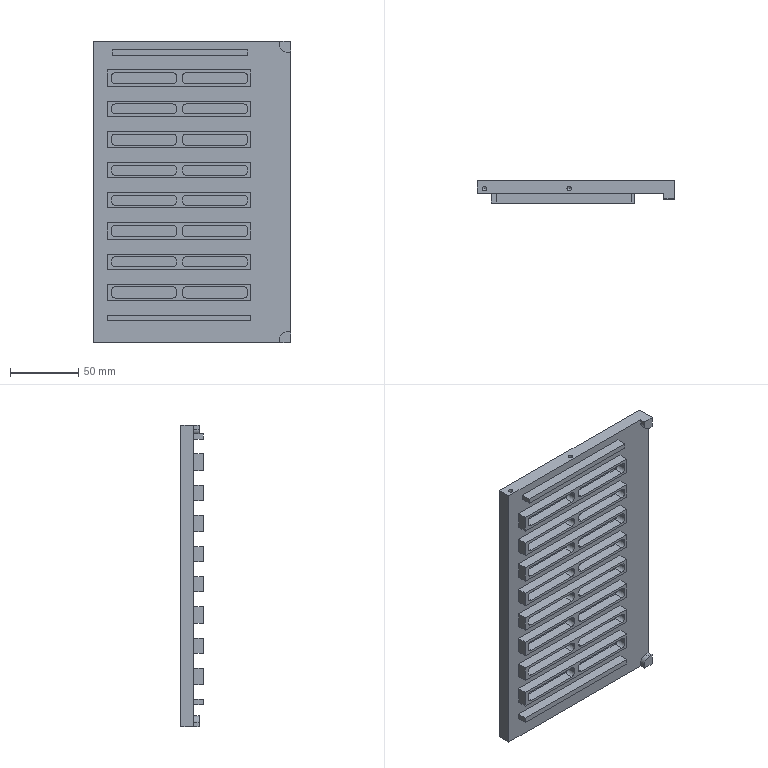Part | 1 solid | 294 faces | box 144.5 x 16.5 x 221 mm | volume 129869 mm3 | plane 176 | cylinder 110 | cone 8 | commonest cylinder face diameters 6 x84 4 x16 3.3 x8 10 x2